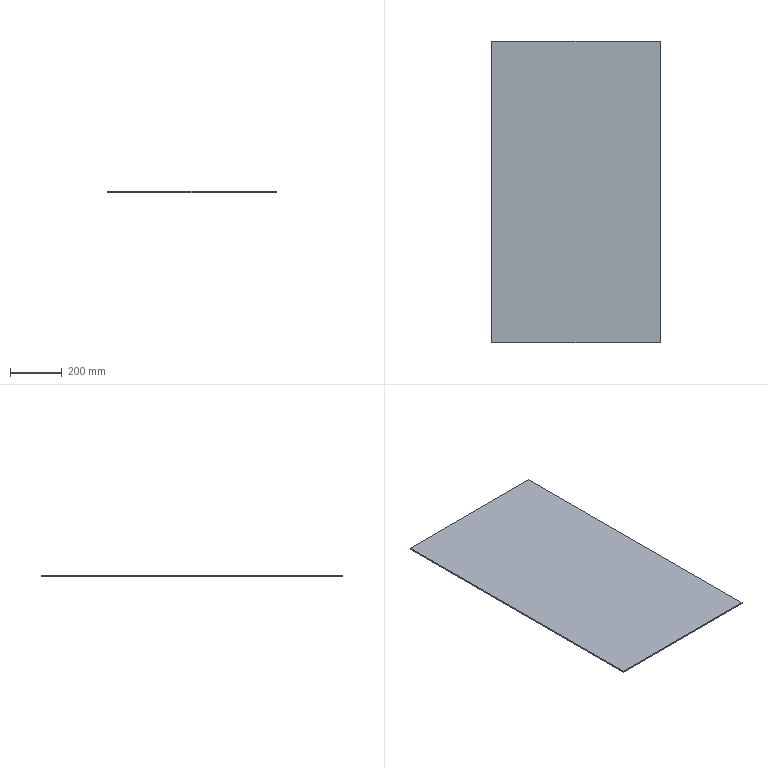Part | SolidWorks | features BaseBody 1, ICE 1 | 1 solid | 6 faces | box 647 x 1160 x 5 mm | volume 3752600 mm3 | plane 6
STEP:
#1=CARTESIAN_POINT('',(87.,1800.,-395.));
#2=VERTEX_POINT('',#1);
#3=CARTESIAN_POINT('',(87.,640.,-395.));
#4=VERTEX_POINT('',#3);
#5=CARTESIAN_POINT('',(87.,1800.,-395.));
#6=DIRECTION('',(0.,-1.,0.));
#7=VECTOR('',#6,1000.);
#8=LINE('',#5,#7);
#9=EDGE_CURVE('',#2,#4,#8,.T.);
#10=ORIENTED_EDGE('',*,*,#9,.F.);
#11=CARTESIAN_POINT('',(-560.,1800.,-395.));
#12=VERTEX_POINT('',#11);
#13=CARTESIAN_POINT('',(-560.,1800.,-395.));
#14=DIRECTION('',(1.,0.,0.));
#15=VECTOR('',#14,1000.);
#16=LINE('',#13,#15);
#17=EDGE_CURVE('',#12,#2,#16,.T.);
#18=ORIENTED_EDGE('',*,*,#17,.F.);
#19=CARTESIAN_POINT('',(-560.,640.,-395.));
#20=VERTEX_POINT('',#19);
#21=CARTESIAN_POINT('',(-560.,640.,-395.));
#22=DIRECTION('',(0.,1.,0.));
#23=VECTOR('',#22,1000.);
#24=LINE('',#21,#23);
#25=EDGE_CURVE('',#20,#12,#24,.T.);
#26=ORIENTED_EDGE('',*,*,#25,.F.);
#27=CARTESIAN_POINT('',(560.,640.,-395.));
#28=DIRECTION('',(-1.,0.,0.));
#29=VECTOR('',#28,1000.);
#30=LINE('',#27,#29);
#31=EDGE_CURVE('',#4,#20,#30,.T.);
#32=ORIENTED_EDGE('',*,*,#31,.F.);
#33=EDGE_LOOP('',(#10,#18,#26,#32));
#34=FACE_OUTER_BOUND('',#33,.T.);
#35=CARTESIAN_POINT('',(0.,1220.,-395.));
#36=DIRECTION('',(0.,0.,1.));
#37=DIRECTION('',(1.,0.,0.));
#38=AXIS2_PLACEMENT_3D('',#35,#36,#37);
#39=PLANE('',#38);
#40=ADVANCED_FACE('',(#34),#39,.T.);
#41=CARTESIAN_POINT('',(87.,640.,-400.));
#42=VERTEX_POINT('',#41);
#43=CARTESIAN_POINT('',(87.,1800.,-400.));
#44=VERTEX_POINT('',#43);
#45=CARTESIAN_POINT('',(87.,1220.,-400.));
#46=DIRECTION('',(0.,1.,0.));
#47=VECTOR('',#46,1000.);
#48=LINE('',#45,#47);
#49=EDGE_CURVE('',#42,#44,#48,.T.);
#50=ORIENTED_EDGE('',*,*,#49,.F.);
#51=CARTESIAN_POINT('',(-560.,640.,-400.));
#52=VERTEX_POINT('',#51);
#53=CARTESIAN_POINT('',(-560.,640.,-400.));
#54=DIRECTION('',(1.,0.,0.));
#55=VECTOR('',#54,1000.);
#56=LINE('',#53,#55);
#57=EDGE_CURVE('',#52,#42,#56,.T.);
#58=ORIENTED_EDGE('',*,*,#57,.F.);
#59=CARTESIAN_POINT('',(-560.,1800.,-400.));
#60=VERTEX_POINT('',#59);
#61=CARTESIAN_POINT('',(-560.,1800.,-400.));
#62=DIRECTION('',(0.,-1.,0.));
#63=VECTOR('',#62,1000.);
#64=LINE('',#61,#63);
#65=EDGE_CURVE('',#60,#52,#64,.T.);
#66=ORIENTED_EDGE('',*,*,#65,.F.);
#67=CARTESIAN_POINT('',(560.,1800.,-400.));
#68=DIRECTION('',(-1.,0.,0.));
#69=VECTOR('',#68,1000.);
#70=LINE('',#67,#69);
#71=EDGE_CURVE('',#44,#60,#70,.T.);
#72=ORIENTED_EDGE('',*,*,#71,.F.);
#73=EDGE_LOOP('',(#50,#58,#66,#72));
#74=FACE_OUTER_BOUND('',#73,.T.);
#75=CARTESIAN_POINT('',(0.,1220.,-400.));
#76=DIRECTION('',(0.,0.,-1.));
#77=DIRECTION('',(0.,-1.,0.));
#78=AXIS2_PLACEMENT_3D('',#75,#76,#77);
#79=PLANE('',#78);
#80=ADVANCED_FACE('',(#74),#79,.T.);
#81=CARTESIAN_POINT('',(87.,640.,-405.));
#82=DIRECTION('',(0.,0.,1.));
#83=VECTOR('',#82,1000.);
#84=LINE('',#81,#83);
#85=EDGE_CURVE('',#42,#4,#84,.T.);
#86=ORIENTED_EDGE('',*,*,#85,.T.);
#87=ORIENTED_EDGE('',*,*,#31,.T.);
#88=CARTESIAN_POINT('',(-560.,640.,-400.));
#89=DIRECTION('',(0.,0.,1.));
#90=VECTOR('',#89,1000.);
#91=LINE('',#88,#90);
#92=EDGE_CURVE('',#52,#20,#91,.T.);
#93=ORIENTED_EDGE('',*,*,#92,.F.);
#94=ORIENTED_EDGE('',*,*,#57,.T.);
#95=EDGE_LOOP('',(#86,#87,#93,#94));
#96=FACE_OUTER_BOUND('',#95,.T.);
#97=CARTESIAN_POINT('',(-560.,640.,-400.));
#98=DIRECTION('',(0.,-1.,0.));
#99=DIRECTION('',(0.,0.,-1.));
#100=AXIS2_PLACEMENT_3D('',#97,#98,#99);
#101=PLANE('',#100);
#102=ADVANCED_FACE('',(#96),#101,.T.);
#103=CARTESIAN_POINT('',(87.,1800.,-400.));
#104=DIRECTION('',(0.,0.,1.));
#105=VECTOR('',#104,1000.);
#106=LINE('',#103,#105);
#107=EDGE_CURVE('',#44,#2,#106,.T.);
#108=ORIENTED_EDGE('',*,*,#107,.F.);
#109=ORIENTED_EDGE('',*,*,#71,.T.);
#110=CARTESIAN_POINT('',(-560.,1800.,-395.));
#111=DIRECTION('',(0.,0.,-1.));
#112=VECTOR('',#111,1000.);
#113=LINE('',#110,#112);
#114=EDGE_CURVE('',#12,#60,#113,.T.);
#115=ORIENTED_EDGE('',*,*,#114,.F.);
#116=ORIENTED_EDGE('',*,*,#17,.T.);
#117=EDGE_LOOP('',(#108,#109,#115,#116));
#118=FACE_OUTER_BOUND('',#117,.T.);
#119=CARTESIAN_POINT('',(560.,1800.,-400.));
#120=DIRECTION('',(0.,1.,0.));
#121=DIRECTION('',(1.,0.,0.));
#122=AXIS2_PLACEMENT_3D('',#119,#120,#121);
#123=PLANE('',#122);
#124=ADVANCED_FACE('',(#118),#123,.T.);
#125=ORIENTED_EDGE('',*,*,#65,.T.);
#126=ORIENTED_EDGE('',*,*,#92,.T.);
#127=ORIENTED_EDGE('',*,*,#25,.T.);
#128=ORIENTED_EDGE('',*,*,#114,.T.);
#129=EDGE_LOOP('',(#125,#126,#127,#128));
#130=FACE_OUTER_BOUND('',#129,.T.);
#131=CARTESIAN_POINT('',(-560.,1800.,-400.));
#132=DIRECTION('',(-1.,0.,0.));
#133=DIRECTION('',(0.,0.,1.));
#134=AXIS2_PLACEMENT_3D('',#131,#132,#133);
#135=PLANE('',#134);
#136=ADVANCED_FACE('',(#130),#135,.T.);
#137=ORIENTED_EDGE('',*,*,#49,.T.);
#138=ORIENTED_EDGE('',*,*,#107,.T.);
#139=ORIENTED_EDGE('',*,*,#9,.T.);
#140=ORIENTED_EDGE('',*,*,#85,.F.);
#141=EDGE_LOOP('',(#137,#138,#139,#140));
#142=FACE_OUTER_BOUND('',#141,.T.);
#143=CARTESIAN_POINT('',(87.,1800.,-405.));
#144=DIRECTION('',(-1.,0.,0.));
#145=DIRECTION('',(0.,0.,1.));
#146=AXIS2_PLACEMENT_3D('',#143,#144,#145);
#147=PLANE('',#146);
#148=ADVANCED_FACE('',(#142),#147,.F.);
#149=CLOSED_SHELL('',(#40,#80,#102,#124,#136,#148));
#150=MANIFOLD_SOLID_BREP('',#149);
#151=CARTESIAN_POINT('',(0.,0.,0.));
#152=DIRECTION('',(0.,0.,1.));
#153=DIRECTION('',(1.,0.,0.));
#154=AXIS2_PLACEMENT_3D('',#151,#152,#153);
#155=(LENGTH_UNIT()NAMED_UNIT(*)SI_UNIT(.MILLI.,.METRE.));
#156=UNCERTAINTY_MEASURE_WITH_UNIT(LENGTH_MEASURE(0.00001),#155,'','');
#157=(NAMED_UNIT(*)PLANE_ANGLE_UNIT()SI_UNIT($,.RADIAN.));
#158=(NAMED_UNIT(*)SI_UNIT($,.STERADIAN.)SOLID_ANGLE_UNIT());
#159=(GEOMETRIC_REPRESENTATION_CONTEXT(3)GLOBAL_UNCERTAINTY_ASSIGNED_CONTEXT((#156))GLOBAL_UNIT_ASSIGNED_CONTEXT((#155,#157,#158))REPRESENTATION_CONTEXT('',''));
#160=ADVANCED_BREP_SHAPE_REPRESENTATION('',(#150,#154),#159);